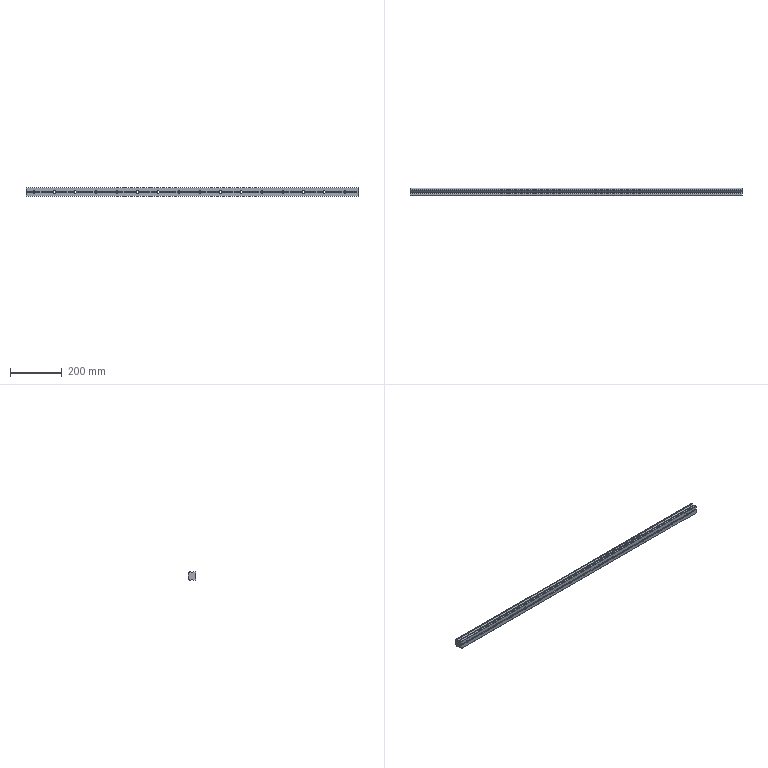Part | STEP file | HWH35HA1080 | 1 solid | 166 faces | box 1280 x 29 x 34 mm | volume 1077935 mm3 | plane 88 | cylinder 78 | commonest cylinder face diameters 9 x32 14 x32 1 x12 18 x2